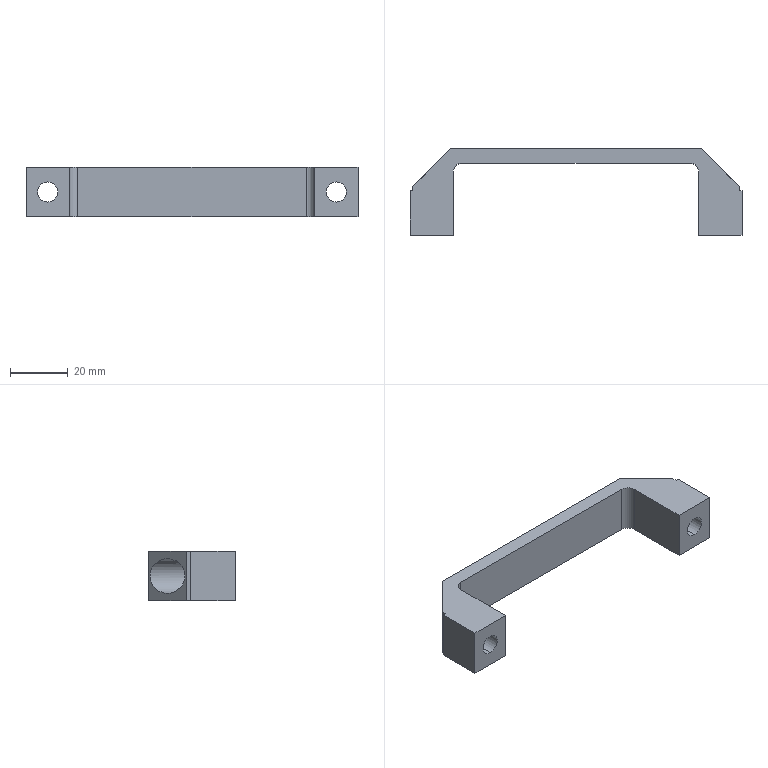Part | STEP file | XAB57-L100 | 1 solid | 32 faces | box 115 x 30 x 17 mm | volume 14990 mm3 | plane 18 | cylinder 10 | cone 4 | commonest cylinder face diameters 7 x4 12 x4 6 x2
STEP:
#1=CARTESIAN_POINT('',(-50.,8.,-6.));
#2=VERTEX_POINT('',#1);
#3=CARTESIAN_POINT('',(-50.,8.,6.));
#4=VERTEX_POINT('',#3);
#5=CARTESIAN_POINT('',(-50.,8.,0.));
#6=DIRECTION('',(0.,1.,0.));
#7=DIRECTION('',(0.,0.,1.));
#8=AXIS2_PLACEMENT_3D('',#5,#6,#7);
#9=CIRCLE('',#8,6.);
#10=EDGE_CURVE('',#2,#4,#9,.T.);
#11=ORIENTED_EDGE('',*,*,#10,.F.);
#12=CARTESIAN_POINT('',(-50.,23.5,-6.));
#13=VERTEX_POINT('',#12);
#14=CARTESIAN_POINT('',(-50.,-50.,-6.));
#15=DIRECTION('',(0.,1.,0.));
#16=VECTOR('',#15,1000.);
#17=LINE('',#14,#16);
#18=EDGE_CURVE('',#2,#13,#17,.T.);
#19=ORIENTED_EDGE('',*,*,#18,.T.);
#20=CARTESIAN_POINT('',(-50.,23.5,6.));
#21=VERTEX_POINT('',#20);
#22=CARTESIAN_POINT('',(-50.,23.5,-6.));
#23=CARTESIAN_POINT('',(-62.,11.5,-6.));
#24=CARTESIAN_POINT('',(-62.,11.5,6.));
#25=CARTESIAN_POINT('',(-50.,23.5,6.));
#26=(BOUNDED_CURVE()B_SPLINE_CURVE(3,(#22,#23,#24,#25),.UNSPECIFIED.,.F.,.F.)B_SPLINE_CURVE_WITH_KNOTS((4,4),(1.571,4.712),.UNSPECIFIED.)CURVE()GEOMETRIC_REPRESENTATION_ITEM()RATIONAL_B_SPLINE_CURVE((1.,0.3333,0.3333,1.))REPRESENTATION_ITEM(''));
#27=EDGE_CURVE('',#13,#21,#26,.T.);
#28=ORIENTED_EDGE('',*,*,#27,.T.);
#29=CARTESIAN_POINT('',(-50.,-50.,6.));
#30=DIRECTION('',(0.,1.,0.));
#31=VECTOR('',#30,1000.);
#32=LINE('',#29,#31);
#33=EDGE_CURVE('',#4,#21,#32,.T.);
#34=ORIENTED_EDGE('',*,*,#33,.F.);
#35=EDGE_LOOP('',(#11,#19,#28,#34));
#36=FACE_OUTER_BOUND('',#35,.T.);
#37=CARTESIAN_POINT('',(-50.,-50.,0.));
#38=DIRECTION('',(0.,1.,0.));
#39=DIRECTION('',(0.,0.,1.));
#40=AXIS2_PLACEMENT_3D('',#37,#38,#39);
#41=CYLINDRICAL_SURFACE('',#40,6.);
#42=ADVANCED_FACE('',(#36),#41,.F.);
#43=CARTESIAN_POINT('',(50.,23.5,-6.));
#44=VERTEX_POINT('',#43);
#45=CARTESIAN_POINT('',(50.,23.5,6.));
#46=VERTEX_POINT('',#45);
#47=CARTESIAN_POINT('',(50.,23.5,-6.));
#48=CARTESIAN_POINT('',(38.,35.5,-6.));
#49=CARTESIAN_POINT('',(38.,35.5,6.));
#50=CARTESIAN_POINT('',(50.,23.5,6.));
#51=(BOUNDED_CURVE()B_SPLINE_CURVE(3,(#47,#48,#49,#50),.UNSPECIFIED.,.F.,.F.)B_SPLINE_CURVE_WITH_KNOTS((4,4),(1.571,4.712),.UNSPECIFIED.)CURVE()GEOMETRIC_REPRESENTATION_ITEM()RATIONAL_B_SPLINE_CURVE((1.,0.3333,0.3333,1.))REPRESENTATION_ITEM(''));
#52=EDGE_CURVE('',#44,#46,#51,.T.);
#53=ORIENTED_EDGE('',*,*,#52,.T.);
#54=CARTESIAN_POINT('',(50.,8.,6.));
#55=VERTEX_POINT('',#54);
#56=CARTESIAN_POINT('',(50.,50.,6.));
#57=DIRECTION('',(0.,-1.,0.));
#58=VECTOR('',#57,1000.);
#59=LINE('',#56,#58);
#60=EDGE_CURVE('',#46,#55,#59,.T.);
#61=ORIENTED_EDGE('',*,*,#60,.T.);
#62=CARTESIAN_POINT('',(50.,8.,-6.));
#63=VERTEX_POINT('',#62);
#64=CARTESIAN_POINT('',(50.,8.,0.));
#65=DIRECTION('',(0.,1.,0.));
#66=DIRECTION('',(0.,0.,-1.));
#67=AXIS2_PLACEMENT_3D('',#64,#65,#66);
#68=CIRCLE('',#67,6.);
#69=EDGE_CURVE('',#63,#55,#68,.T.);
#70=ORIENTED_EDGE('',*,*,#69,.F.);
#71=CARTESIAN_POINT('',(50.,50.,-6.));
#72=DIRECTION('',(0.,-1.,0.));
#73=VECTOR('',#72,1000.);
#74=LINE('',#71,#73);
#75=EDGE_CURVE('',#44,#63,#74,.T.);
#76=ORIENTED_EDGE('',*,*,#75,.F.);
#77=EDGE_LOOP('',(#53,#61,#70,#76));
#78=FACE_OUTER_BOUND('',#77,.T.);
#79=CARTESIAN_POINT('',(50.,50.,0.));
#80=DIRECTION('',(0.,-1.,0.));
#81=DIRECTION('',(0.,0.,-1.));
#82=AXIS2_PLACEMENT_3D('',#79,#80,#81);
#83=CYLINDRICAL_SURFACE('',#82,6.);
#84=ADVANCED_FACE('',(#78),#83,.F.);
#85=CARTESIAN_POINT('',(50.,7.,3.5));
#86=VERTEX_POINT('',#85);
#87=CARTESIAN_POINT('',(50.,7.,-3.5));
#88=VERTEX_POINT('',#87);
#89=CARTESIAN_POINT('',(50.,7.,0.));
#90=DIRECTION('',(0.,-1.,0.));
#91=DIRECTION('',(0.,0.,-1.));
#92=AXIS2_PLACEMENT_3D('',#89,#90,#91);
#93=CIRCLE('',#92,3.5);
#94=EDGE_CURVE('',#86,#88,#93,.T.);
#95=ORIENTED_EDGE('',*,*,#94,.F.);
#96=CARTESIAN_POINT('',(50.,0.,3.5));
#97=VERTEX_POINT('',#96);
#98=CARTESIAN_POINT('',(50.,50.,3.5));
#99=DIRECTION('',(0.,-1.,0.));
#100=VECTOR('',#99,1000.);
#101=LINE('',#98,#100);
#102=EDGE_CURVE('',#86,#97,#101,.T.);
#103=ORIENTED_EDGE('',*,*,#102,.T.);
#104=CARTESIAN_POINT('',(50.,0.,-3.5));
#105=VERTEX_POINT('',#104);
#106=CARTESIAN_POINT('',(50.,0.,0.));
#107=DIRECTION('',(0.,-1.,0.));
#108=DIRECTION('',(0.,0.,-1.));
#109=AXIS2_PLACEMENT_3D('',#106,#107,#108);
#110=CIRCLE('',#109,3.5);
#111=EDGE_CURVE('',#97,#105,#110,.T.);
#112=ORIENTED_EDGE('',*,*,#111,.T.);
#113=CARTESIAN_POINT('',(50.,50.,-3.5));
#114=DIRECTION('',(0.,-1.,0.));
#115=VECTOR('',#114,1000.);
#116=LINE('',#113,#115);
#117=EDGE_CURVE('',#88,#105,#116,.T.);
#118=ORIENTED_EDGE('',*,*,#117,.F.);
#119=EDGE_LOOP('',(#95,#103,#112,#118));
#120=FACE_OUTER_BOUND('',#119,.T.);
#121=CARTESIAN_POINT('',(50.,50.,0.));
#122=DIRECTION('',(0.,-1.,0.));
#123=DIRECTION('',(0.,0.,-1.));
#124=AXIS2_PLACEMENT_3D('',#121,#122,#123);
#125=CYLINDRICAL_SURFACE('',#124,3.5);
#126=ADVANCED_FACE('',(#120),#125,.F.);
#127=CARTESIAN_POINT('',(-50.,0.,3.5));
#128=VERTEX_POINT('',#127);
#129=CARTESIAN_POINT('',(-50.,0.,-3.5));
#130=VERTEX_POINT('',#129);
#131=CARTESIAN_POINT('',(-50.,0.,0.));
#132=DIRECTION('',(0.,-1.,0.));
#133=DIRECTION('',(0.,0.,1.));
#134=AXIS2_PLACEMENT_3D('',#131,#132,#133);
#135=CIRCLE('',#134,3.5);
#136=EDGE_CURVE('',#128,#130,#135,.T.);
#137=ORIENTED_EDGE('',*,*,#136,.T.);
#138=CARTESIAN_POINT('',(-50.,7.,-3.5));
#139=VERTEX_POINT('',#138);
#140=CARTESIAN_POINT('',(-50.,-50.,-3.5));
#141=DIRECTION('',(0.,1.,0.));
#142=VECTOR('',#141,1000.);
#143=LINE('',#140,#142);
#144=EDGE_CURVE('',#130,#139,#143,.T.);
#145=ORIENTED_EDGE('',*,*,#144,.T.);
#146=CARTESIAN_POINT('',(-50.,7.,3.5));
#147=VERTEX_POINT('',#146);
#148=CARTESIAN_POINT('',(-50.,7.,0.));
#149=DIRECTION('',(0.,-1.,0.));
#150=DIRECTION('',(0.,0.,1.));
#151=AXIS2_PLACEMENT_3D('',#148,#149,#150);
#152=CIRCLE('',#151,3.5);
#153=EDGE_CURVE('',#147,#139,#152,.T.);
#154=ORIENTED_EDGE('',*,*,#153,.F.);
#155=CARTESIAN_POINT('',(-50.,-50.,3.5));
#156=DIRECTION('',(0.,1.,0.));
#157=VECTOR('',#156,1000.);
#158=LINE('',#155,#157);
#159=EDGE_CURVE('',#128,#147,#158,.T.);
#160=ORIENTED_EDGE('',*,*,#159,.F.);
#161=EDGE_LOOP('',(#137,#145,#154,#160));
#162=FACE_OUTER_BOUND('',#161,.T.);
#163=CARTESIAN_POINT('',(-50.,-50.,0.));
#164=DIRECTION('',(0.,1.,0.));
#165=DIRECTION('',(0.,0.,1.));
#166=AXIS2_PLACEMENT_3D('',#163,#164,#165);
#167=CYLINDRICAL_SURFACE('',#166,3.5);
#168=ADVANCED_FACE('',(#162),#167,.F.);
#169=CARTESIAN_POINT('',(-50.,7.,-5.));
#170=VERTEX_POINT('',#169);
#171=CARTESIAN_POINT('',(-50.,7.,5.));
#172=VERTEX_POINT('',#171);
#173=CARTESIAN_POINT('',(-50.,7.,0.));
#174=DIRECTION('',(0.,1.,0.));
#175=DIRECTION('',(0.,0.,1.));
#176=AXIS2_PLACEMENT_3D('',#173,#174,#175);
#177=CIRCLE('',#176,5.);
#178=EDGE_CURVE('',#170,#172,#177,.T.);
#179=ORIENTED_EDGE('',*,*,#178,.F.);
#180=CARTESIAN_POINT('',(-50.,8.,-6.));
#181=DIRECTION('',(0.,0.7071,-0.7071));
#182=VECTOR('',#181,1000.);
#183=LINE('',#180,#182);
#184=EDGE_CURVE('',#170,#2,#183,.T.);
#185=ORIENTED_EDGE('',*,*,#184,.T.);
#186=ORIENTED_EDGE('',*,*,#10,.T.);
#187=CARTESIAN_POINT('',(-50.,8.,6.));
#188=DIRECTION('',(0.,0.7071,0.7071));
#189=VECTOR('',#188,1000.);
#190=LINE('',#187,#189);
#191=EDGE_CURVE('',#172,#4,#190,.T.);
#192=ORIENTED_EDGE('',*,*,#191,.F.);
#193=EDGE_LOOP('',(#179,#185,#186,#192));
#194=FACE_OUTER_BOUND('',#193,.T.);
#195=CARTESIAN_POINT('',(-50.,8.,0.));
#196=DIRECTION('',(0.,1.,0.));
#197=DIRECTION('',(0.,0.,1.));
#198=AXIS2_PLACEMENT_3D('',#195,#196,#197);
#199=CONICAL_SURFACE('',#198,6.,0.7854);
#200=ADVANCED_FACE('',(#194),#199,.F.);
#201=CARTESIAN_POINT('',(50.,7.,-5.));
#202=VERTEX_POINT('',#201);
#203=CARTESIAN_POINT('',(50.,7.,5.));
#204=VERTEX_POINT('',#203);
#205=CARTESIAN_POINT('',(50.,7.,0.));
#206=DIRECTION('',(0.,1.,0.));
#207=DIRECTION('',(0.,0.,1.));
#208=AXIS2_PLACEMENT_3D('',#205,#206,#207);
#209=CIRCLE('',#208,5.);
#210=EDGE_CURVE('',#202,#204,#209,.T.);
#211=ORIENTED_EDGE('',*,*,#210,.F.);
#212=CARTESIAN_POINT('',(50.,8.,-6.));
#213=DIRECTION('',(0.,0.7071,-0.7071));
#214=VECTOR('',#213,1000.);
#215=LINE('',#212,#214);
#216=EDGE_CURVE('',#202,#63,#215,.T.);
#217=ORIENTED_EDGE('',*,*,#216,.T.);
#218=ORIENTED_EDGE('',*,*,#69,.T.);
#219=CARTESIAN_POINT('',(50.,8.,6.));
#220=DIRECTION('',(0.,0.7071,0.7071));
#221=VECTOR('',#220,1000.);
#222=LINE('',#219,#221);
#223=EDGE_CURVE('',#204,#55,#222,.T.);
#224=ORIENTED_EDGE('',*,*,#223,.F.);
#225=EDGE_LOOP('',(#211,#217,#218,#224));
#226=FACE_OUTER_BOUND('',#225,.T.);
#227=CARTESIAN_POINT('',(50.,8.,0.));
#228=DIRECTION('',(0.,1.,0.));
#229=DIRECTION('',(0.,0.,1.));
#230=AXIS2_PLACEMENT_3D('',#227,#228,#229);
#231=CONICAL_SURFACE('',#230,6.,0.7854);
#232=ADVANCED_FACE('',(#226),#231,.F.);
#233=CARTESIAN_POINT('',(-43.5,30.,8.5));
#234=VERTEX_POINT('',#233);
#235=CARTESIAN_POINT('',(-43.5,30.,-8.5));
#236=VERTEX_POINT('',#235);
#237=CARTESIAN_POINT('',(-43.5,30.,8.5));
#238=DIRECTION('',(0.,0.,-1.));
#239=VECTOR('',#238,1000.);
#240=LINE('',#237,#239);
#241=EDGE_CURVE('',#234,#236,#240,.T.);
#242=ORIENTED_EDGE('',*,*,#241,.F.);
#243=CARTESIAN_POINT('',(43.5,30.,8.5));
#244=VERTEX_POINT('',#243);
#245=CARTESIAN_POINT('',(43.5,30.,8.5));
#246=DIRECTION('',(-1.,0.,0.));
#247=VECTOR('',#246,1000.);
#248=LINE('',#245,#247);
#249=EDGE_CURVE('',#244,#234,#248,.T.);
#250=ORIENTED_EDGE('',*,*,#249,.F.);
#251=CARTESIAN_POINT('',(43.5,30.,-8.5));
#252=VERTEX_POINT('',#251);
#253=CARTESIAN_POINT('',(43.5,30.,8.5));
#254=DIRECTION('',(0.,0.,1.));
#255=VECTOR('',#254,1000.);
#256=LINE('',#253,#255);
#257=EDGE_CURVE('',#252,#244,#256,.T.);
#258=ORIENTED_EDGE('',*,*,#257,.F.);
#259=CARTESIAN_POINT('',(43.5,30.,-8.5));
#260=DIRECTION('',(1.,0.,0.));
#261=VECTOR('',#260,1000.);
#262=LINE('',#259,#261);
#263=EDGE_CURVE('',#236,#252,#262,.T.);
#264=ORIENTED_EDGE('',*,*,#263,.F.);
#265=EDGE_LOOP('',(#242,#250,#258,#264));
#266=FACE_OUTER_BOUND('',#265,.T.);
#267=CARTESIAN_POINT('',(43.5,30.,8.5));
#268=DIRECTION('',(0.,-1.,0.));
#269=DIRECTION('',(0.,0.,-1.));
#270=AXIS2_PLACEMENT_3D('',#267,#268,#269);
#271=PLANE('',#270);
#272=ADVANCED_FACE('',(#266),#271,.F.);
#273=CARTESIAN_POINT('',(-56.5,15.5,-8.5));
#274=VERTEX_POINT('',#273);
#275=CARTESIAN_POINT('',(-56.5,17.,-8.5));
#276=VERTEX_POINT('',#275);
#277=CARTESIAN_POINT('',(-56.5,17.,-8.5));
#278=DIRECTION('',(0.,1.,0.));
#279=VECTOR('',#278,1000.);
#280=LINE('',#277,#279);
#281=EDGE_CURVE('',#274,#276,#280,.T.);
#282=ORIENTED_EDGE('',*,*,#281,.T.);
#283=CARTESIAN_POINT('',(-43.5,30.,-8.5));
#284=DIRECTION('',(-0.7071,-0.7071,0.));
#285=VECTOR('',#284,1000.);
#286=LINE('',#283,#285);
#287=EDGE_CURVE('',#236,#276,#286,.T.);
#288=ORIENTED_EDGE('',*,*,#287,.F.);
#289=ORIENTED_EDGE('',*,*,#263,.T.);
#290=CARTESIAN_POINT('',(56.5,17.,-8.5));
#291=VERTEX_POINT('',#290);
#292=CARTESIAN_POINT('',(56.5,17.,-8.5));
#293=DIRECTION('',(-0.7071,0.7071,0.));
#294=VECTOR('',#293,1000.);
#295=LINE('',#292,#294);
#296=EDGE_CURVE('',#291,#252,#295,.T.);
#297=ORIENTED_EDGE('',*,*,#296,.F.);
#298=CARTESIAN_POINT('',(56.5,15.5,-8.5));
#299=VERTEX_POINT('',#298);
#300=CARTESIAN_POINT('',(56.5,15.5,-8.5));
#301=DIRECTION('',(0.,-1.,0.));
#302=VECTOR('',#301,1000.);
#303=LINE('',#300,#302);
#304=EDGE_CURVE('',#291,#299,#303,.T.);
#305=ORIENTED_EDGE('',*,*,#304,.T.);
#306=CARTESIAN_POINT('',(57.5,15.5,-8.5));
#307=VERTEX_POINT('',#306);
#308=CARTESIAN_POINT('',(57.5,15.5,-8.5));
#309=DIRECTION('',(1.,0.,0.));
#310=VECTOR('',#309,1000.);
#311=LINE('',#308,#310);
#312=EDGE_CURVE('',#299,#307,#311,.T.);
#313=ORIENTED_EDGE('',*,*,#312,.T.);
#314=CARTESIAN_POINT('',(57.5,0.,-8.5));
#315=VERTEX_POINT('',#314);
#316=CARTESIAN_POINT('',(57.5,22.,-8.5));
#317=DIRECTION('',(0.,1.,0.));
#318=VECTOR('',#317,1000.);
#319=LINE('',#316,#318);
#320=EDGE_CURVE('',#315,#307,#319,.T.);
#321=ORIENTED_EDGE('',*,*,#320,.F.);
#322=CARTESIAN_POINT('',(42.5,0.,-8.5));
#323=VERTEX_POINT('',#322);
#324=CARTESIAN_POINT('',(-39.5,0.,-8.5));
#325=DIRECTION('',(1.,0.,0.));
#326=VECTOR('',#325,1000.);
#327=LINE('',#324,#326);
#328=EDGE_CURVE('',#323,#315,#327,.T.);
#329=ORIENTED_EDGE('',*,*,#328,.F.);
#330=CARTESIAN_POINT('',(42.5,22.,-8.5));
#331=VERTEX_POINT('',#330);
#332=CARTESIAN_POINT('',(42.5,22.,-8.5));
#333=DIRECTION('',(0.,-1.,0.));
#334=VECTOR('',#333,1000.);
#335=LINE('',#332,#334);
#336=EDGE_CURVE('',#331,#323,#335,.T.);
#337=ORIENTED_EDGE('',*,*,#336,.F.);
#338=CARTESIAN_POINT('',(39.5,25.,-8.5));
#339=VERTEX_POINT('',#338);
#340=CARTESIAN_POINT('',(39.5,22.,-8.5));
#341=DIRECTION('',(0.,0.,-1.));
#342=DIRECTION('',(1.,0.,0.));
#343=AXIS2_PLACEMENT_3D('',#340,#341,#342);
#344=CIRCLE('',#343,3.);
#345=EDGE_CURVE('',#339,#331,#344,.T.);
#346=ORIENTED_EDGE('',*,*,#345,.F.);
#347=CARTESIAN_POINT('',(-39.5,25.,-8.5));
#348=VERTEX_POINT('',#347);
#349=CARTESIAN_POINT('',(-39.5,25.,-8.5));
#350=DIRECTION('',(1.,0.,0.));
#351=VECTOR('',#350,1000.);
#352=LINE('',#349,#351);
#353=EDGE_CURVE('',#348,#339,#352,.T.);
#354=ORIENTED_EDGE('',*,*,#353,.F.);
#355=CARTESIAN_POINT('',(-42.5,22.,-8.5));
#356=VERTEX_POINT('',#355);
#357=CARTESIAN_POINT('',(-39.5,22.,-8.5));
#358=DIRECTION('',(0.,0.,-1.));
#359=DIRECTION('',(1.,0.,0.));
#360=AXIS2_PLACEMENT_3D('',#357,#358,#359);
#361=CIRCLE('',#360,3.);
#362=EDGE_CURVE('',#356,#348,#361,.T.);
#363=ORIENTED_EDGE('',*,*,#362,.F.);
#364=CARTESIAN_POINT('',(-42.5,0.,-8.5));
#365=VERTEX_POINT('',#364);
#366=CARTESIAN_POINT('',(-42.5,22.,-8.5));
#367=DIRECTION('',(0.,1.,0.));
#368=VECTOR('',#367,1000.);
#369=LINE('',#366,#368);
#370=EDGE_CURVE('',#365,#356,#369,.T.);
#371=ORIENTED_EDGE('',*,*,#370,.F.);
#372=CARTESIAN_POINT('',(-57.5,0.,-8.5));
#373=VERTEX_POINT('',#372);
#374=CARTESIAN_POINT('',(-39.5,0.,-8.5));
#375=DIRECTION('',(1.,0.,0.));
#376=VECTOR('',#375,1000.);
#377=LINE('',#374,#376);
#378=EDGE_CURVE('',#373,#365,#377,.T.);
#379=ORIENTED_EDGE('',*,*,#378,.F.);
#380=CARTESIAN_POINT('',(-57.5,15.5,-8.5));
#381=VERTEX_POINT('',#380);
#382=CARTESIAN_POINT('',(-57.5,22.,-8.5));
#383=DIRECTION('',(0.,-1.,0.));
#384=VECTOR('',#383,1000.);
#385=LINE('',#382,#384);
#386=EDGE_CURVE('',#381,#373,#385,.T.);
#387=ORIENTED_EDGE('',*,*,#386,.F.);
#388=CARTESIAN_POINT('',(-56.5,15.5,-8.5));
#389=DIRECTION('',(1.,0.,0.));
#390=VECTOR('',#389,1000.);
#391=LINE('',#388,#390);
#392=EDGE_CURVE('',#381,#274,#391,.T.);
#393=ORIENTED_EDGE('',*,*,#392,.T.);
#394=EDGE_LOOP('',(#282,#288,#289,#297,#305,#313,#321,#329,#337,#346,#354,#363,#371,#379,#387,#393));
#395=FACE_OUTER_BOUND('',#394,.T.);
#396=CARTESIAN_POINT('',(-39.5,22.,-8.5));
#397=DIRECTION('',(0.,0.,1.));
#398=DIRECTION('',(1.,0.,0.));
#399=AXIS2_PLACEMENT_3D('',#396,#397,#398);
#400=PLANE('',#399);
#401=ADVANCED_FACE('',(#395),#400,.F.);
#402=CARTESIAN_POINT('',(-56.5,17.,8.5));
#403=VERTEX_POINT('',#402);
#404=CARTESIAN_POINT('',(-56.5,17.,8.5));
#405=DIRECTION('',(0.,0.,-1.));
#406=VECTOR('',#405,1000.);
#407=LINE('',#404,#406);
#408=EDGE_CURVE('',#403,#276,#407,.T.);
#409=ORIENTED_EDGE('',*,*,#408,.F.);
#410=CARTESIAN_POINT('',(-43.5,30.,8.5));
#411=DIRECTION('',(-0.7071,-0.7071,0.));
#412=VECTOR('',#411,1000.);
#413=LINE('',#410,#412);
#414=EDGE_CURVE('',#234,#403,#413,.T.);
#415=ORIENTED_EDGE('',*,*,#414,.F.);
#416=ORIENTED_EDGE('',*,*,#241,.T.);
#417=ORIENTED_EDGE('',*,*,#287,.T.);
#418=EDGE_LOOP('',(#409,#415,#416,#417));
#419=FACE_OUTER_BOUND('',#418,.T.);
#420=CARTESIAN_POINT('',(-50.,23.5,6.));
#421=CARTESIAN_POINT('',(-38.,35.5,6.));
#422=CARTESIAN_POINT('',(-38.,35.5,-6.));
#423=CARTESIAN_POINT('',(-50.,23.5,-6.));
#424=(BOUNDED_CURVE()B_SPLINE_CURVE(3,(#420,#421,#422,#423),.UNSPECIFIED.,.F.,.F.)B_SPLINE_CURVE_WITH_KNOTS((4,4),(4.712,7.854),.UNSPECIFIED.)CURVE()GEOMETRIC_REPRESENTATION_ITEM()RATIONAL_B_SPLINE_CURVE((1.,0.3333,0.3333,1.))REPRESENTATION_ITEM(''));
#425=EDGE_CURVE('',#21,#13,#424,.T.);
#426=ORIENTED_EDGE('',*,*,#425,.F.);
#427=ORIENTED_EDGE('',*,*,#27,.F.);
#428=EDGE_LOOP('',(#426,#427));
#429=FACE_BOUND('',#428,.T.);
#430=CARTESIAN_POINT('',(-43.5,30.,8.5));
#431=DIRECTION('',(0.7071,-0.7071,0.));
#432=DIRECTION('',(0.7071,0.7071,0.));
#433=AXIS2_PLACEMENT_3D('',#430,#431,#432);
#434=PLANE('',#433);
#435=ADVANCED_FACE('',(#419,#429),#434,.F.);
#436=ORIENTED_EDGE('',*,*,#414,.T.);
#437=CARTESIAN_POINT('',(-56.5,15.5,8.5));
#438=VERTEX_POINT('',#437);
#439=CARTESIAN_POINT('',(-56.5,22.,8.5));
#440=DIRECTION('',(0.,-1.,0.));
#441=VECTOR('',#440,1000.);
#442=LINE('',#439,#441);
#443=EDGE_CURVE('',#403,#438,#442,.T.);
#444=ORIENTED_EDGE('',*,*,#443,.T.);
#445=CARTESIAN_POINT('',(-57.5,15.5,8.5));
#446=VERTEX_POINT('',#445);
#447=CARTESIAN_POINT('',(-56.5,15.5,8.5));
#448=DIRECTION('',(-1.,0.,0.));
#449=VECTOR('',#448,1000.);
#450=LINE('',#447,#449);
#451=EDGE_CURVE('',#438,#446,#450,.T.);
#452=ORIENTED_EDGE('',*,*,#451,.T.);
#453=CARTESIAN_POINT('',(-57.5,0.,8.5));
#454=VERTEX_POINT('',#453);
#455=CARTESIAN_POINT('',(-57.5,22.,8.5));
#456=DIRECTION('',(0.,-1.,0.));
#457=VECTOR('',#456,1000.);
#458=LINE('',#455,#457);
#459=EDGE_CURVE('',#446,#454,#458,.T.);
#460=ORIENTED_EDGE('',*,*,#459,.T.);
#461=CARTESIAN_POINT('',(-42.5,0.,8.5));
#462=VERTEX_POINT('',#461);
#463=CARTESIAN_POINT('',(-39.5,0.,8.5));
#464=DIRECTION('',(1.,0.,0.));
#465=VECTOR('',#464,1000.);
#466=LINE('',#463,#465);
#467=EDGE_CURVE('',#454,#462,#466,.T.);
#468=ORIENTED_EDGE('',*,*,#467,.T.);
#469=CARTESIAN_POINT('',(-42.5,22.,8.5));
#470=VERTEX_POINT('',#469);
#471=CARTESIAN_POINT('',(-42.5,22.,8.5));
#472=DIRECTION('',(0.,1.,0.));
#473=VECTOR('',#472,1000.);
#474=LINE('',#471,#473);
#475=EDGE_CURVE('',#462,#470,#474,.T.);
#476=ORIENTED_EDGE('',*,*,#475,.T.);
#477=CARTESIAN_POINT('',(-39.5,25.,8.5));
#478=VERTEX_POINT('',#477);
#479=CARTESIAN_POINT('',(-39.5,22.,8.5));
#480=DIRECTION('',(0.,0.,-1.));
#481=DIRECTION('',(1.,0.,0.));
#482=AXIS2_PLACEMENT_3D('',#479,#480,#481);
#483=CIRCLE('',#482,3.);
#484=EDGE_CURVE('',#470,#478,#483,.T.);
#485=ORIENTED_EDGE('',*,*,#484,.T.);
#486=CARTESIAN_POINT('',(39.5,25.,8.5));
#487=VERTEX_POINT('',#486);
#488=CARTESIAN_POINT('',(-39.5,25.,8.5));
#489=DIRECTION('',(1.,0.,0.));
#490=VECTOR('',#489,1000.);
#491=LINE('',#488,#490);
#492=EDGE_CURVE('',#478,#487,#491,.T.);
#493=ORIENTED_EDGE('',*,*,#492,.T.);
#494=CARTESIAN_POINT('',(42.5,22.,8.5));
#495=VERTEX_POINT('',#494);
#496=CARTESIAN_POINT('',(39.5,22.,8.5));
#497=DIRECTION('',(0.,0.,-1.));
#498=DIRECTION('',(1.,0.,0.));
#499=AXIS2_PLACEMENT_3D('',#496,#497,#498);
#500=CIRCLE('',#499,3.);
#501=EDGE_CURVE('',#487,#495,#500,.T.);
#502=ORIENTED_EDGE('',*,*,#501,.T.);
#503=CARTESIAN_POINT('',(42.5,0.,8.5));
#504=VERTEX_POINT('',#503);
#505=CARTESIAN_POINT('',(42.5,22.,8.5));
#506=DIRECTION('',(0.,-1.,0.));
#507=VECTOR('',#506,1000.);
#508=LINE('',#505,#507);
#509=EDGE_CURVE('',#495,#504,#508,.T.);
#510=ORIENTED_EDGE('',*,*,#509,.T.);
#511=CARTESIAN_POINT('',(57.5,0.,8.5));
#512=VERTEX_POINT('',#511);
#513=CARTESIAN_POINT('',(-39.5,0.,8.5));
#514=DIRECTION('',(1.,0.,0.));
#515=VECTOR('',#514,1000.);
#516=LINE('',#513,#515);
#517=EDGE_CURVE('',#504,#512,#516,.T.);
#518=ORIENTED_EDGE('',*,*,#517,.T.);
#519=CARTESIAN_POINT('',(57.5,15.5,8.5));
#520=VERTEX_POINT('',#519);
#521=CARTESIAN_POINT('',(57.5,22.,8.5));
#522=DIRECTION('',(0.,1.,0.));
#523=VECTOR('',#522,1000.);
#524=LINE('',#521,#523);
#525=EDGE_CURVE('',#512,#520,#524,.T.);
#526=ORIENTED_EDGE('',*,*,#525,.T.);
#527=CARTESIAN_POINT('',(56.5,15.5,8.5));
#528=VERTEX_POINT('',#527);
#529=CARTESIAN_POINT('',(57.5,15.5,8.5));
#530=DIRECTION('',(-1.,0.,0.));
#531=VECTOR('',#530,1000.);
#532=LINE('',#529,#531);
#533=EDGE_CURVE('',#520,#528,#532,.T.);
#534=ORIENTED_EDGE('',*,*,#533,.T.);
#535=CARTESIAN_POINT('',(56.5,17.,8.5));
#536=VERTEX_POINT('',#535);
#537=CARTESIAN_POINT('',(56.5,15.5,8.5));
#538=DIRECTION('',(0.,1.,0.));
#539=VECTOR('',#538,1000.);
#540=LINE('',#537,#539);
#541=EDGE_CURVE('',#528,#536,#540,.T.);
#542=ORIENTED_EDGE('',*,*,#541,.T.);
#543=CARTESIAN_POINT('',(56.5,17.,8.5));
#544=DIRECTION('',(-0.7071,0.7071,0.));
#545=VECTOR('',#544,1000.);
#546=LINE('',#543,#545);
#547=EDGE_CURVE('',#536,#244,#546,.T.);
#548=ORIENTED_EDGE('',*,*,#547,.T.);
#549=ORIENTED_EDGE('',*,*,#249,.T.);
#550=EDGE_LOOP('',(#436,#444,#452,#460,#468,#476,#485,#493,#502,#510,#518,#526,#534,#542,#548,#549));
#551=FACE_OUTER_BOUND('',#550,.T.);
#552=CARTESIAN_POINT('',(-39.5,22.,8.5));
#553=DIRECTION('',(0.,0.,1.));
#554=DIRECTION('',(1.,0.,0.));
#555=AXIS2_PLACEMENT_3D('',#552,#553,#554);
#556=PLANE('',#555);
#557=ADVANCED_FACE('',(#551),#556,.T.);
#558=ORIENTED_EDGE('',*,*,#257,.T.);
#559=ORIENTED_EDGE('',*,*,#547,.F.);
#560=CARTESIAN_POINT('',(56.5,17.,8.5));
#561=DIRECTION('',(0.,0.,1.));
#562=VECTOR('',#561,1000.);
#563=LINE('',#560,#562);
#564=EDGE_CURVE('',#291,#536,#563,.T.);
#565=ORIENTED_EDGE('',*,*,#564,.F.);
#566=ORIENTED_EDGE('',*,*,#296,.T.);
#567=EDGE_LOOP('',(#558,#559,#565,#566));
#568=FACE_OUTER_BOUND('',#567,.T.);
#569=ORIENTED_EDGE('',*,*,#52,.F.);
#570=CARTESIAN_POINT('',(50.,23.5,6.));
#571=CARTESIAN_POINT('',(62.,11.5,6.));
#572=CARTESIAN_POINT('',(62.,11.5,-6.));
#573=CARTESIAN_POINT('',(50.,23.5,-6.));
#574=(BOUNDED_CURVE()B_SPLINE_CURVE(3,(#570,#571,#572,#573),.UNSPECIFIED.,.F.,.F.)B_SPLINE_CURVE_WITH_KNOTS((4,4),(4.712,7.854),.UNSPECIFIED.)CURVE()GEOMETRIC_REPRESENTATION_ITEM()RATIONAL_B_SPLINE_CURVE((1.,0.3333,0.3333,1.))REPRESENTATION_ITEM(''));
#575=EDGE_CURVE('',#46,#44,#574,.T.);
#576=ORIENTED_EDGE('',*,*,#575,.F.);
#577=EDGE_LOOP('',(#569,#576));
#578=FACE_BOUND('',#577,.T.);
#579=CARTESIAN_POINT('',(56.5,17.,8.5));
#580=DIRECTION('',(-0.7071,-0.7071,0.));
#581=DIRECTION('',(0.7071,-0.7071,0.));
#582=AXIS2_PLACEMENT_3D('',#579,#580,#581);
#583=PLANE('',#582);
#584=ADVANCED_FACE('',(#568,#578),#583,.F.);
#585=CARTESIAN_POINT('',(57.5,15.5,8.5));
#586=DIRECTION('',(0.,0.,-1.));
#587=VECTOR('',#586,1000.);
#588=LINE('',#585,#587);
#589=EDGE_CURVE('',#520,#307,#588,.T.);
#590=ORIENTED_EDGE('',*,*,#589,.F.);
#591=ORIENTED_EDGE('',*,*,#525,.F.);
#592=CARTESIAN_POINT('',(57.5,0.,8.5));
#593=DIRECTION('',(0.,0.,1.));
#594=VECTOR('',#593,1000.);
#595=LINE('',#592,#594);
#596=EDGE_CURVE('',#315,#512,#595,.T.);
#597=ORIENTED_EDGE('',*,*,#596,.F.);
#598=ORIENTED_EDGE('',*,*,#320,.T.);
#599=EDGE_LOOP('',(#590,#591,#597,#598));
#600=FACE_OUTER_BOUND('',#599,.T.);
#601=CARTESIAN_POINT('',(57.5,0.,8.5));
#602=DIRECTION('',(-1.,0.,0.));
#603=DIRECTION('',(0.,0.,1.));
#604=AXIS2_PLACEMENT_3D('',#601,#602,#603);
#605=PLANE('',#604);
#606=ADVANCED_FACE('',(#600),#605,.F.);
#607=ORIENTED_EDGE('',*,*,#596,.T.);
#608=ORIENTED_EDGE('',*,*,#517,.F.);
#609=CARTESIAN_POINT('',(42.5,0.,8.5));
#610=DIRECTION('',(0.,0.,1.));
#611=VECTOR('',#610,1000.);
#612=LINE('',#609,#611);
#613=EDGE_CURVE('',#323,#504,#612,.T.);
#614=ORIENTED_EDGE('',*,*,#613,.F.);
#615=ORIENTED_EDGE('',*,*,#328,.T.);
#616=EDGE_LOOP('',(#607,#608,#614,#615));
#617=FACE_OUTER_BOUND('',#616,.T.);
#618=CARTESIAN_POINT('',(50.,0.,0.));
#619=DIRECTION('',(0.,-1.,0.));
#620=DIRECTION('',(0.,0.,-1.));
#621=AXIS2_PLACEMENT_3D('',#618,#619,#620);
#622=CIRCLE('',#621,3.5);
#623=EDGE_CURVE('',#105,#97,#622,.T.);
#624=ORIENTED_EDGE('',*,*,#623,.F.);
#625=ORIENTED_EDGE('',*,*,#111,.F.);
#626=EDGE_LOOP('',(#624,#625));
#627=FACE_BOUND('',#626,.T.);
#628=CARTESIAN_POINT('',(42.5,0.,8.5));
#629=DIRECTION('',(0.,1.,0.));
#630=DIRECTION('',(0.,0.,1.));
#631=AXIS2_PLACEMENT_3D('',#628,#629,#630);
#632=PLANE('',#631);
#633=ADVANCED_FACE('',(#617,#627),#632,.F.);
#634=ORIENTED_EDGE('',*,*,#613,.T.);
#635=ORIENTED_EDGE('',*,*,#509,.F.);
#636=CARTESIAN_POINT('',(42.5,22.,8.5));
#637=DIRECTION('',(0.,0.,1.));
#638=VECTOR('',#637,1000.);
#639=LINE('',#636,#638);
#640=EDGE_CURVE('',#331,#495,#639,.T.);
#641=ORIENTED_EDGE('',*,*,#640,.F.);
#642=ORIENTED_EDGE('',*,*,#336,.T.);
#643=EDGE_LOOP('',(#634,#635,#641,#642));
#644=FACE_OUTER_BOUND('',#643,.T.);
#645=CARTESIAN_POINT('',(42.5,22.,8.5));
#646=DIRECTION('',(1.,0.,0.));
#647=DIRECTION('',(0.,0.,-1.));
#648=AXIS2_PLACEMENT_3D('',#645,#646,#647);
#649=PLANE('',#648);
#650=ADVANCED_FACE('',(#644),#649,.F.);
#651=ORIENTED_EDGE('',*,*,#640,.T.);
#652=ORIENTED_EDGE('',*,*,#501,.F.);
#653=CARTESIAN_POINT('',(39.5,25.,8.5));
#654=DIRECTION('',(0.,0.,1.));
#655=VECTOR('',#654,1000.);
#656=LINE('',#653,#655);
#657=EDGE_CURVE('',#339,#487,#656,.T.);
#658=ORIENTED_EDGE('',*,*,#657,.F.);
#659=ORIENTED_EDGE('',*,*,#345,.T.);
#660=EDGE_LOOP('',(#651,#652,#658,#659));
#661=FACE_OUTER_BOUND('',#660,.T.);
#662=CARTESIAN_POINT('',(39.5,22.,8.5));
#663=DIRECTION('',(0.,0.,1.));
#664=DIRECTION('',(1.,0.,0.));
#665=AXIS2_PLACEMENT_3D('',#662,#663,#664);
#666=CYLINDRICAL_SURFACE('',#665,3.);
#667=ADVANCED_FACE('',(#661),#666,.F.);
#668=ORIENTED_EDGE('',*,*,#657,.T.);
#669=ORIENTED_EDGE('',*,*,#492,.F.);
#670=CARTESIAN_POINT('',(-39.5,25.,8.5));
#671=DIRECTION('',(0.,0.,1.));
#672=VECTOR('',#671,1000.);
#673=LINE('',#670,#672);
#674=EDGE_CURVE('',#348,#478,#673,.T.);
#675=ORIENTED_EDGE('',*,*,#674,.F.);
#676=ORIENTED_EDGE('',*,*,#353,.T.);
#677=EDGE_LOOP('',(#668,#669,#675,#676));
#678=FACE_OUTER_BOUND('',#677,.T.);
#679=CARTESIAN_POINT('',(-39.5,25.,8.5));
#680=DIRECTION('',(0.,1.,0.));
#681=DIRECTION('',(0.,0.,1.));
#682=AXIS2_PLACEMENT_3D('',#679,#680,#681);
#683=PLANE('',#682);
#684=ADVANCED_FACE('',(#678),#683,.F.);
#685=ORIENTED_EDGE('',*,*,#674,.T.);
#686=ORIENTED_EDGE('',*,*,#484,.F.);
#687=CARTESIAN_POINT('',(-42.5,22.,8.5));
#688=DIRECTION('',(0.,0.,1.));
#689=VECTOR('',#688,1000.);
#690=LINE('',#687,#689);
#691=EDGE_CURVE('',#356,#470,#690,.T.);
#692=ORIENTED_EDGE('',*,*,#691,.F.);
#693=ORIENTED_EDGE('',*,*,#362,.T.);
#694=EDGE_LOOP('',(#685,#686,#692,#693));
#695=FACE_OUTER_BOUND('',#694,.T.);
#696=CARTESIAN_POINT('',(-39.5,22.,8.5));
#697=DIRECTION('',(0.,0.,1.));
#698=DIRECTION('',(1.,0.,0.));
#699=AXIS2_PLACEMENT_3D('',#696,#697,#698);
#700=CYLINDRICAL_SURFACE('',#699,3.);
#701=ADVANCED_FACE('',(#695),#700,.F.);
#702=ORIENTED_EDGE('',*,*,#691,.T.);
#703=ORIENTED_EDGE('',*,*,#475,.F.);
#704=CARTESIAN_POINT('',(-42.5,0.,8.5));
#705=DIRECTION('',(0.,0.,1.));
#706=VECTOR('',#705,1000.);
#707=LINE('',#704,#706);
#708=EDGE_CURVE('',#365,#462,#707,.T.);
#709=ORIENTED_EDGE('',*,*,#708,.F.);
#710=ORIENTED_EDGE('',*,*,#370,.T.);
#711=EDGE_LOOP('',(#702,#703,#709,#710));
#712=FACE_OUTER_BOUND('',#711,.T.);
#713=CARTESIAN_POINT('',(-42.5,0.,8.5));
#714=DIRECTION('',(-1.,0.,0.));
#715=DIRECTION('',(0.,0.,1.));
#716=AXIS2_PLACEMENT_3D('',#713,#714,#715);
#717=PLANE('',#716);
#718=ADVANCED_FACE('',(#712),#717,.F.);
#719=ORIENTED_EDGE('',*,*,#708,.T.);
#720=ORIENTED_EDGE('',*,*,#467,.F.);
#721=CARTESIAN_POINT('',(-57.5,0.,8.5));
#722=DIRECTION('',(0.,0.,1.));
#723=VECTOR('',#722,1000.);
#724=LINE('',#721,#723);
#725=EDGE_CURVE('',#373,#454,#724,.T.);
#726=ORIENTED_EDGE('',*,*,#725,.F.);
#727=ORIENTED_EDGE('',*,*,#378,.T.);
#728=EDGE_LOOP('',(#719,#720,#726,#727));
#729=FACE_OUTER_BOUND('',#728,.T.);
#730=ORIENTED_EDGE('',*,*,#136,.F.);
#731=CARTESIAN_POINT('',(-50.,0.,0.));
#732=DIRECTION('',(0.,-1.,0.));
#733=DIRECTION('',(0.,0.,1.));
#734=AXIS2_PLACEMENT_3D('',#731,#732,#733);
#735=CIRCLE('',#734,3.5);
#736=EDGE_CURVE('',#130,#128,#735,.T.);
#737=ORIENTED_EDGE('',*,*,#736,.F.);
#738=EDGE_LOOP('',(#730,#737));
#739=FACE_BOUND('',#738,.T.);
#740=CARTESIAN_POINT('',(-57.5,0.,8.5));
#741=DIRECTION('',(0.,1.,0.));
#742=DIRECTION('',(0.,0.,1.));
#743=AXIS2_PLACEMENT_3D('',#740,#741,#742);
#744=PLANE('',#743);
#745=ADVANCED_FACE('',(#729,#739),#744,.F.);
#746=ORIENTED_EDGE('',*,*,#725,.T.);
#747=ORIENTED_EDGE('',*,*,#459,.F.);
#748=CARTESIAN_POINT('',(-57.5,15.5,8.5));
#749=DIRECTION('',(0.,0.,1.));
#750=VECTOR('',#749,1000.);
#751=LINE('',#748,#750);
#752=EDGE_CURVE('',#381,#446,#751,.T.);
#753=ORIENTED_EDGE('',*,*,#752,.F.);
#754=ORIENTED_EDGE('',*,*,#386,.T.);
#755=EDGE_LOOP('',(#746,#747,#753,#754));
#756=FACE_OUTER_BOUND('',#755,.T.);
#757=CARTESIAN_POINT('',(-57.5,15.5,8.5));
#758=DIRECTION('',(1.,0.,0.));
#759=DIRECTION('',(0.,0.,-1.));
#760=AXIS2_PLACEMENT_3D('',#757,#758,#759);
#761=PLANE('',#760);
#762=ADVANCED_FACE('',(#756),#761,.F.);
#763=CARTESIAN_POINT('',(-56.5,15.5,8.5));
#764=DIRECTION('',(0.,0.,-1.));
#765=VECTOR('',#764,1000.);
#766=LINE('',#763,#765);
#767=EDGE_CURVE('',#438,#274,#766,.T.);
#768=ORIENTED_EDGE('',*,*,#767,.F.);
#769=ORIENTED_EDGE('',*,*,#443,.F.);
#770=ORIENTED_EDGE('',*,*,#408,.T.);
#771=ORIENTED_EDGE('',*,*,#281,.F.);
#772=EDGE_LOOP('',(#768,#769,#770,#771));
#773=FACE_OUTER_BOUND('',#772,.T.);
#774=CARTESIAN_POINT('',(-56.5,17.,8.5));
#775=DIRECTION('',(1.,0.,0.));
#776=DIRECTION('',(0.,0.,-1.));
#777=AXIS2_PLACEMENT_3D('',#774,#775,#776);
#778=PLANE('',#777);
#779=ADVANCED_FACE('',(#773),#778,.F.);
#780=ORIENTED_EDGE('',*,*,#18,.F.);
#781=CARTESIAN_POINT('',(-50.,8.,0.));
#782=DIRECTION('',(0.,1.,0.));
#783=DIRECTION('',(0.,0.,1.));
#784=AXIS2_PLACEMENT_3D('',#781,#782,#783);
#785=CIRCLE('',#784,6.);
#786=EDGE_CURVE('',#4,#2,#785,.T.);
#787=ORIENTED_EDGE('',*,*,#786,.F.);
#788=ORIENTED_EDGE('',*,*,#33,.T.);
#789=ORIENTED_EDGE('',*,*,#425,.T.);
#790=EDGE_LOOP('',(#780,#787,#788,#789));
#791=FACE_OUTER_BOUND('',#790,.T.);
#792=CARTESIAN_POINT('',(-50.,-50.,0.));
#793=DIRECTION('',(0.,1.,0.));
#794=DIRECTION('',(0.,0.,1.));
#795=AXIS2_PLACEMENT_3D('',#792,#793,#794);
#796=CYLINDRICAL_SURFACE('',#795,6.);
#797=ADVANCED_FACE('',(#791),#796,.F.);
#798=ORIENTED_EDGE('',*,*,#564,.T.);
#799=ORIENTED_EDGE('',*,*,#541,.F.);
#800=CARTESIAN_POINT('',(56.5,15.5,8.5));
#801=DIRECTION('',(0.,0.,1.));
#802=VECTOR('',#801,1000.);
#803=LINE('',#800,#802);
#804=EDGE_CURVE('',#299,#528,#803,.T.);
#805=ORIENTED_EDGE('',*,*,#804,.F.);
#806=ORIENTED_EDGE('',*,*,#304,.F.);
#807=EDGE_LOOP('',(#798,#799,#805,#806));
#808=FACE_OUTER_BOUND('',#807,.T.);
#809=CARTESIAN_POINT('',(56.5,15.5,8.5));
#810=DIRECTION('',(-1.,0.,0.));
#811=DIRECTION('',(0.,0.,1.));
#812=AXIS2_PLACEMENT_3D('',#809,#810,#811);
#813=PLANE('',#812);
#814=ADVANCED_FACE('',(#808),#813,.F.);
#815=ORIENTED_EDGE('',*,*,#60,.F.);
#816=ORIENTED_EDGE('',*,*,#575,.T.);
#817=ORIENTED_EDGE('',*,*,#75,.T.);
#818=CARTESIAN_POINT('',(50.,8.,0.));
#819=DIRECTION('',(0.,1.,0.));
#820=DIRECTION('',(0.,0.,-1.));
#821=AXIS2_PLACEMENT_3D('',#818,#819,#820);
#822=CIRCLE('',#821,6.);
#823=EDGE_CURVE('',#55,#63,#822,.T.);
#824=ORIENTED_EDGE('',*,*,#823,.F.);
#825=EDGE_LOOP('',(#815,#816,#817,#824));
#826=FACE_OUTER_BOUND('',#825,.T.);
#827=CARTESIAN_POINT('',(50.,50.,0.));
#828=DIRECTION('',(0.,-1.,0.));
#829=DIRECTION('',(0.,0.,-1.));
#830=AXIS2_PLACEMENT_3D('',#827,#828,#829);
#831=CYLINDRICAL_SURFACE('',#830,6.);
#832=ADVANCED_FACE('',(#826),#831,.F.);
#833=ORIENTED_EDGE('',*,*,#804,.T.);
#834=ORIENTED_EDGE('',*,*,#533,.F.);
#835=ORIENTED_EDGE('',*,*,#589,.T.);
#836=ORIENTED_EDGE('',*,*,#312,.F.);
#837=EDGE_LOOP('',(#833,#834,#835,#836));
#838=FACE_OUTER_BOUND('',#837,.T.);
#839=CARTESIAN_POINT('',(57.5,15.5,8.5));
#840=DIRECTION('',(0.,-1.,0.));
#841=DIRECTION('',(0.,0.,-1.));
#842=AXIS2_PLACEMENT_3D('',#839,#840,#841);
#843=PLANE('',#842);
#844=ADVANCED_FACE('',(#838),#843,.F.);
#845=ORIENTED_EDGE('',*,*,#102,.F.);
#846=CARTESIAN_POINT('',(50.,7.,0.));
#847=DIRECTION('',(0.,-1.,0.));
#848=DIRECTION('',(0.,0.,-1.));
#849=AXIS2_PLACEMENT_3D('',#846,#847,#848);
#850=CIRCLE('',#849,3.5);
#851=EDGE_CURVE('',#88,#86,#850,.T.);
#852=ORIENTED_EDGE('',*,*,#851,.F.);
#853=ORIENTED_EDGE('',*,*,#117,.T.);
#854=ORIENTED_EDGE('',*,*,#623,.T.);
#855=EDGE_LOOP('',(#845,#852,#853,#854));
#856=FACE_OUTER_BOUND('',#855,.T.);
#857=CARTESIAN_POINT('',(50.,50.,0.));
#858=DIRECTION('',(0.,-1.,0.));
#859=DIRECTION('',(0.,0.,-1.));
#860=AXIS2_PLACEMENT_3D('',#857,#858,#859);
#861=CYLINDRICAL_SURFACE('',#860,3.5);
#862=ADVANCED_FACE('',(#856),#861,.F.);
#863=ORIENTED_EDGE('',*,*,#144,.F.);
#864=ORIENTED_EDGE('',*,*,#736,.T.);
#865=ORIENTED_EDGE('',*,*,#159,.T.);
#866=CARTESIAN_POINT('',(-50.,7.,0.));
#867=DIRECTION('',(0.,-1.,0.));
#868=DIRECTION('',(0.,0.,1.));
#869=AXIS2_PLACEMENT_3D('',#866,#867,#868);
#870=CIRCLE('',#869,3.5);
#871=EDGE_CURVE('',#139,#147,#870,.T.);
#872=ORIENTED_EDGE('',*,*,#871,.F.);
#873=EDGE_LOOP('',(#863,#864,#865,#872));
#874=FACE_OUTER_BOUND('',#873,.T.);
#875=CARTESIAN_POINT('',(-50.,-50.,0.));
#876=DIRECTION('',(0.,1.,0.));
#877=DIRECTION('',(0.,0.,1.));
#878=AXIS2_PLACEMENT_3D('',#875,#876,#877);
#879=CYLINDRICAL_SURFACE('',#878,3.5);
#880=ADVANCED_FACE('',(#874),#879,.F.);
#881=ORIENTED_EDGE('',*,*,#752,.T.);
#882=ORIENTED_EDGE('',*,*,#451,.F.);
#883=ORIENTED_EDGE('',*,*,#767,.T.);
#884=ORIENTED_EDGE('',*,*,#392,.F.);
#885=EDGE_LOOP('',(#881,#882,#883,#884));
#886=FACE_OUTER_BOUND('',#885,.T.);
#887=CARTESIAN_POINT('',(-56.5,15.5,8.5));
#888=DIRECTION('',(0.,-1.,0.));
#889=DIRECTION('',(0.,0.,-1.));
#890=AXIS2_PLACEMENT_3D('',#887,#888,#889);
#891=PLANE('',#890);
#892=ADVANCED_FACE('',(#886),#891,.F.);
#893=ORIENTED_EDGE('',*,*,#184,.F.);
#894=CARTESIAN_POINT('',(-50.,7.,0.));
#895=DIRECTION('',(0.,1.,0.));
#896=DIRECTION('',(0.,0.,1.));
#897=AXIS2_PLACEMENT_3D('',#894,#895,#896);
#898=CIRCLE('',#897,5.);
#899=EDGE_CURVE('',#172,#170,#898,.T.);
#900=ORIENTED_EDGE('',*,*,#899,.F.);
#901=ORIENTED_EDGE('',*,*,#191,.T.);
#902=ORIENTED_EDGE('',*,*,#786,.T.);
#903=EDGE_LOOP('',(#893,#900,#901,#902));
#904=FACE_OUTER_BOUND('',#903,.T.);
#905=CARTESIAN_POINT('',(-50.,8.,0.));
#906=DIRECTION('',(0.,1.,0.));
#907=DIRECTION('',(0.,0.,1.));
#908=AXIS2_PLACEMENT_3D('',#905,#906,#907);
#909=CONICAL_SURFACE('',#908,6.,0.7854);
#910=ADVANCED_FACE('',(#904),#909,.F.);
#911=ORIENTED_EDGE('',*,*,#216,.F.);
#912=CARTESIAN_POINT('',(50.,7.,0.));
#913=DIRECTION('',(0.,1.,0.));
#914=DIRECTION('',(0.,0.,1.));
#915=AXIS2_PLACEMENT_3D('',#912,#913,#914);
#916=CIRCLE('',#915,5.);
#917=EDGE_CURVE('',#204,#202,#916,.T.);
#918=ORIENTED_EDGE('',*,*,#917,.F.);
#919=ORIENTED_EDGE('',*,*,#223,.T.);
#920=ORIENTED_EDGE('',*,*,#823,.T.);
#921=EDGE_LOOP('',(#911,#918,#919,#920));
#922=FACE_OUTER_BOUND('',#921,.T.);
#923=CARTESIAN_POINT('',(50.,8.,0.));
#924=DIRECTION('',(0.,1.,0.));
#925=DIRECTION('',(0.,0.,1.));
#926=AXIS2_PLACEMENT_3D('',#923,#924,#925);
#927=CONICAL_SURFACE('',#926,6.,0.7854);
#928=ADVANCED_FACE('',(#922),#927,.F.);
#929=ORIENTED_EDGE('',*,*,#851,.T.);
#930=ORIENTED_EDGE('',*,*,#94,.T.);
#931=EDGE_LOOP('',(#929,#930));
#932=FACE_BOUND('',#931,.T.);
#933=ORIENTED_EDGE('',*,*,#917,.T.);
#934=ORIENTED_EDGE('',*,*,#210,.T.);
#935=EDGE_LOOP('',(#933,#934));
#936=FACE_OUTER_BOUND('',#935,.T.);
#937=CARTESIAN_POINT('',(46.5,7.,0.));
#938=DIRECTION('',(0.,1.,0.));
#939=DIRECTION('',(0.,0.,1.));
#940=AXIS2_PLACEMENT_3D('',#937,#938,#939);
#941=PLANE('',#940);
#942=ADVANCED_FACE('',(#932,#936),#941,.T.);
#943=ORIENTED_EDGE('',*,*,#153,.T.);
#944=ORIENTED_EDGE('',*,*,#871,.T.);
#945=EDGE_LOOP('',(#943,#944));
#946=FACE_BOUND('',#945,.T.);
#947=ORIENTED_EDGE('',*,*,#899,.T.);
#948=ORIENTED_EDGE('',*,*,#178,.T.);
#949=EDGE_LOOP('',(#947,#948));
#950=FACE_OUTER_BOUND('',#949,.T.);
#951=CARTESIAN_POINT('',(-44.,7.,0.));
#952=DIRECTION('',(0.,1.,0.));
#953=DIRECTION('',(0.,0.,1.));
#954=AXIS2_PLACEMENT_3D('',#951,#952,#953);
#955=PLANE('',#954);
#956=ADVANCED_FACE('',(#946,#950),#955,.T.);
#957=CLOSED_SHELL('',(#42,#84,#126,#168,#200,#232,#272,#401,#435,#557,#584,#606,#633,#650,#667,#684,#701,#718,#745,#762,#779,#797,#814,#832,#844,#862,#880,#892,#910,#928,#942,#956));
#958=MANIFOLD_SOLID_BREP('',#957);
#959=CARTESIAN_POINT('',(0.,0.,0.));
#960=DIRECTION('',(0.,0.,1.));
#961=DIRECTION('',(1.,0.,0.));
#962=AXIS2_PLACEMENT_3D('',#959,#960,#961);
#963=(LENGTH_UNIT()NAMED_UNIT(*)SI_UNIT(.MILLI.,.METRE.));
#964=UNCERTAINTY_MEASURE_WITH_UNIT(LENGTH_MEASURE(0.00001),#963,'','');
#965=(NAMED_UNIT(*)PLANE_ANGLE_UNIT()SI_UNIT($,.RADIAN.));
#966=(NAMED_UNIT(*)SI_UNIT($,.STERADIAN.)SOLID_ANGLE_UNIT());
#967=(GEOMETRIC_REPRESENTATION_CONTEXT(3)GLOBAL_UNCERTAINTY_ASSIGNED_CONTEXT((#964))GLOBAL_UNIT_ASSIGNED_CONTEXT((#963,#965,#966))REPRESENTATION_CONTEXT('',''));
#968=ADVANCED_BREP_SHAPE_REPRESENTATION('',(#958,#962),#967);